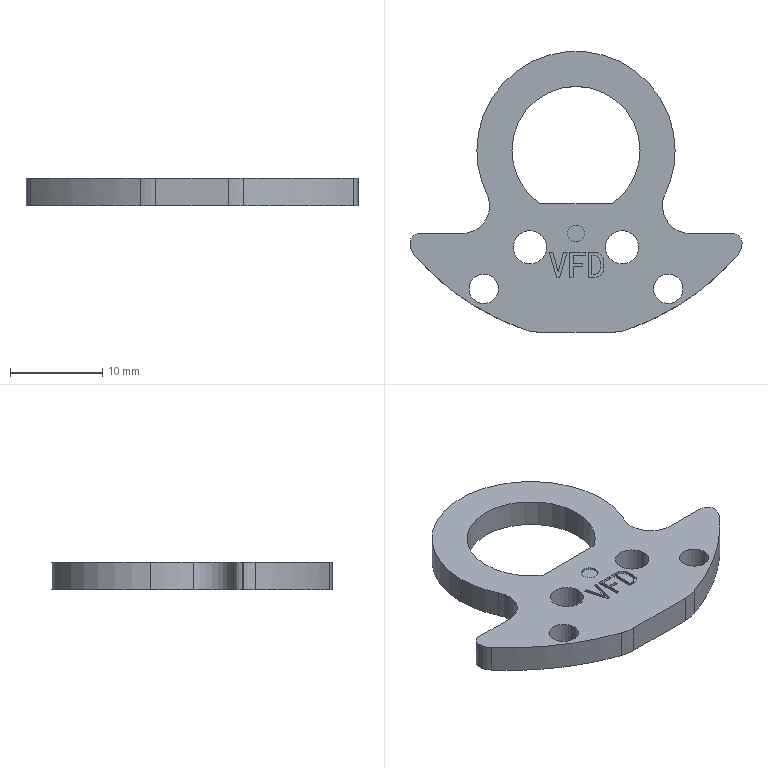Part | SolidWorks | features BaseBody 1 | 1 solid | 72 faces | box 36 x 30.45 x 3 mm | volume 1415 mm3 | plane 37 | cylinder 27 | cone 4 | spline 4 | commonest cylinder face diameters 3.2 x4 3.6 x4 6 x3 13.9 x3 21.5 x3 1.8 x2